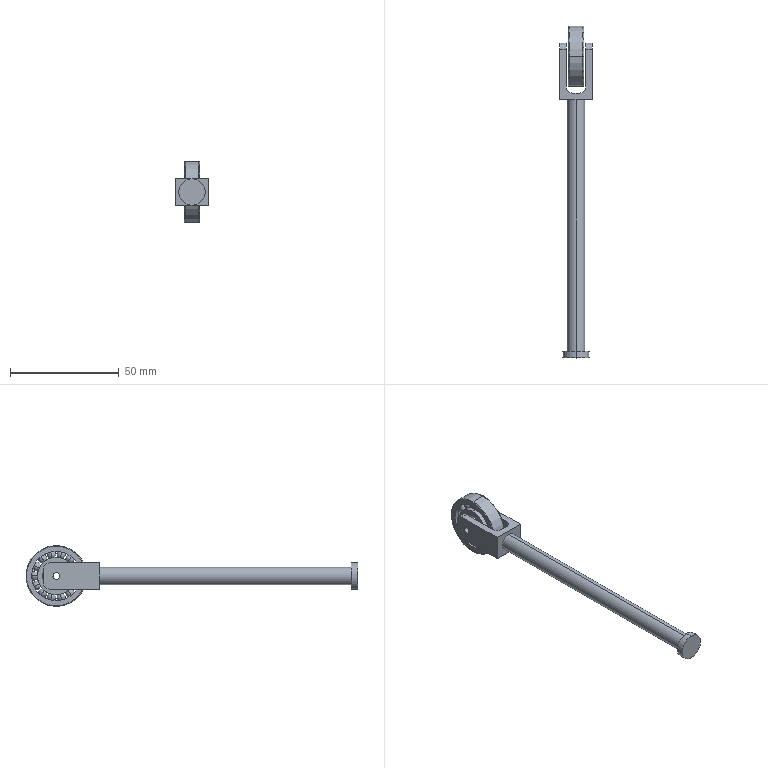Part | SolidWorks | 2 solids | 123 faces | box 15 x 153 x 28 mm | volume 10997 mm3 | torus 53 | sphere 28 | cylinder 26 | plane 16 | commonest cylinder face diameters 6 x6 3 x4 17.333 x4 22.667 x4 8 x2 12 x2